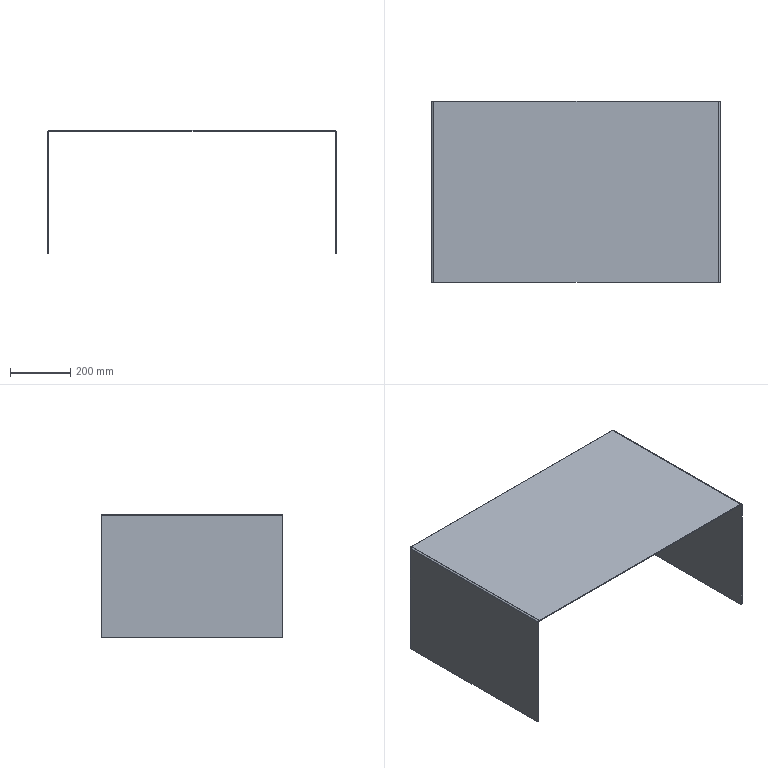Part | SolidWorks | features FlatPattern 1, ICE 1, SMBaseFlange 1, SheetMetal 1 | 1 solid | 26 faces | box 956 x 600 x 410 mm | volume 3179024 mm3 | plane 18 | cylinder 8 | commonest cylinder face diameters 6 x6 12 x2
STEP:
#1=CARTESIAN_POINT('',(956.,0.,-407.));
#2=VERTEX_POINT('',#1);
#3=CARTESIAN_POINT('',(956.,3.,-410.));
#4=VERTEX_POINT('',#3);
#5=CARTESIAN_POINT('',(956.,3.,-407.));
#6=DIRECTION('',(1.,0.,0.));
#7=DIRECTION('',(0.,0.,1.));
#8=AXIS2_PLACEMENT_3D('',#5,#6,#7);
#9=CIRCLE('',#8,3.);
#10=EDGE_CURVE('',#2,#4,#9,.T.);
#11=ORIENTED_EDGE('',*,*,#10,.T.);
#12=CARTESIAN_POINT('',(956.,597.,-410.));
#13=VERTEX_POINT('',#12);
#14=CARTESIAN_POINT('',(956.,600.,-410.));
#15=DIRECTION('',(0.,-1.,0.));
#16=VECTOR('',#15,1000.);
#17=LINE('',#14,#16);
#18=EDGE_CURVE('',#13,#4,#17,.T.);
#19=ORIENTED_EDGE('',*,*,#18,.F.);
#20=CARTESIAN_POINT('',(956.,600.,-407.));
#21=VERTEX_POINT('',#20);
#22=CARTESIAN_POINT('',(956.,597.,-407.));
#23=DIRECTION('',(1.,0.,0.));
#24=DIRECTION('',(0.,0.,1.));
#25=AXIS2_PLACEMENT_3D('',#22,#23,#24);
#26=CIRCLE('',#25,3.);
#27=EDGE_CURVE('',#13,#21,#26,.T.);
#28=ORIENTED_EDGE('',*,*,#27,.T.);
#29=CARTESIAN_POINT('',(956.,600.,-6.));
#30=VERTEX_POINT('',#29);
#31=CARTESIAN_POINT('',(956.,600.,0.));
#32=DIRECTION('',(0.,0.,-1.));
#33=VECTOR('',#32,1000.);
#34=LINE('',#31,#33);
#35=EDGE_CURVE('',#30,#21,#34,.T.);
#36=ORIENTED_EDGE('',*,*,#35,.F.);
#37=CARTESIAN_POINT('',(956.,0.,-6.));
#38=VERTEX_POINT('',#37);
#39=CARTESIAN_POINT('',(956.,600.,-6.));
#40=DIRECTION('',(0.,-1.,0.));
#41=VECTOR('',#40,1000.);
#42=LINE('',#39,#41);
#43=EDGE_CURVE('',#30,#38,#42,.T.);
#44=ORIENTED_EDGE('',*,*,#43,.T.);
#45=CARTESIAN_POINT('',(956.,0.,0.));
#46=DIRECTION('',(0.,0.,-1.));
#47=VECTOR('',#46,1000.);
#48=LINE('',#45,#47);
#49=EDGE_CURVE('',#38,#2,#48,.T.);
#50=ORIENTED_EDGE('',*,*,#49,.T.);
#51=EDGE_LOOP('',(#11,#19,#28,#36,#44,#50));
#52=FACE_OUTER_BOUND('',#51,.T.);
#53=CARTESIAN_POINT('',(956.,600.,0.));
#54=DIRECTION('',(-1.,0.,0.));
#55=DIRECTION('',(0.,0.,1.));
#56=AXIS2_PLACEMENT_3D('',#53,#54,#55);
#57=PLANE('',#56);
#58=ADVANCED_FACE('',(#52),#57,.F.);
#59=CARTESIAN_POINT('',(953.,597.,-410.));
#60=VERTEX_POINT('',#59);
#61=CARTESIAN_POINT('',(953.,3.,-410.));
#62=VERTEX_POINT('',#61);
#63=CARTESIAN_POINT('',(953.,600.,-410.));
#64=DIRECTION('',(0.,-1.,0.));
#65=VECTOR('',#64,1000.);
#66=LINE('',#63,#65);
#67=EDGE_CURVE('',#60,#62,#66,.T.);
#68=ORIENTED_EDGE('',*,*,#67,.T.);
#69=CARTESIAN_POINT('',(953.,0.,-407.));
#70=VERTEX_POINT('',#69);
#71=CARTESIAN_POINT('',(953.,3.,-407.));
#72=DIRECTION('',(1.,0.,0.));
#73=DIRECTION('',(0.,0.,1.));
#74=AXIS2_PLACEMENT_3D('',#71,#72,#73);
#75=CIRCLE('',#74,3.);
#76=EDGE_CURVE('',#70,#62,#75,.T.);
#77=ORIENTED_EDGE('',*,*,#76,.F.);
#78=CARTESIAN_POINT('',(953.,0.,-6.));
#79=VERTEX_POINT('',#78);
#80=CARTESIAN_POINT('',(953.,0.,0.));
#81=DIRECTION('',(0.,0.,-1.));
#82=VECTOR('',#81,1000.);
#83=LINE('',#80,#82);
#84=EDGE_CURVE('',#79,#70,#83,.T.);
#85=ORIENTED_EDGE('',*,*,#84,.F.);
#86=CARTESIAN_POINT('',(953.,600.,-6.));
#87=VERTEX_POINT('',#86);
#88=CARTESIAN_POINT('',(953.,600.,-6.));
#89=DIRECTION('',(0.,-1.,0.));
#90=VECTOR('',#89,1000.);
#91=LINE('',#88,#90);
#92=EDGE_CURVE('',#87,#79,#91,.T.);
#93=ORIENTED_EDGE('',*,*,#92,.F.);
#94=CARTESIAN_POINT('',(953.,600.,-407.));
#95=VERTEX_POINT('',#94);
#96=CARTESIAN_POINT('',(953.,600.,0.));
#97=DIRECTION('',(0.,0.,-1.));
#98=VECTOR('',#97,1000.);
#99=LINE('',#96,#98);
#100=EDGE_CURVE('',#87,#95,#99,.T.);
#101=ORIENTED_EDGE('',*,*,#100,.T.);
#102=CARTESIAN_POINT('',(953.,597.,-407.));
#103=DIRECTION('',(1.,0.,0.));
#104=DIRECTION('',(0.,0.,1.));
#105=AXIS2_PLACEMENT_3D('',#102,#103,#104);
#106=CIRCLE('',#105,3.);
#107=EDGE_CURVE('',#60,#95,#106,.T.);
#108=ORIENTED_EDGE('',*,*,#107,.F.);
#109=EDGE_LOOP('',(#68,#77,#85,#93,#101,#108));
#110=FACE_OUTER_BOUND('',#109,.T.);
#111=CARTESIAN_POINT('',(953.,600.,0.));
#112=DIRECTION('',(-1.,0.,0.));
#113=DIRECTION('',(0.,0.,1.));
#114=AXIS2_PLACEMENT_3D('',#111,#112,#113);
#115=PLANE('',#114);
#116=ADVANCED_FACE('',(#110),#115,.T.);
#117=ORIENTED_EDGE('',*,*,#18,.T.);
#118=CARTESIAN_POINT('',(953.,3.,-410.));
#119=DIRECTION('',(1.,0.,0.));
#120=VECTOR('',#119,1000.);
#121=LINE('',#118,#120);
#122=EDGE_CURVE('',#62,#4,#121,.T.);
#123=ORIENTED_EDGE('',*,*,#122,.F.);
#124=ORIENTED_EDGE('',*,*,#67,.F.);
#125=CARTESIAN_POINT('',(953.,597.,-410.));
#126=DIRECTION('',(1.,0.,0.));
#127=VECTOR('',#126,1000.);
#128=LINE('',#125,#127);
#129=EDGE_CURVE('',#60,#13,#128,.T.);
#130=ORIENTED_EDGE('',*,*,#129,.T.);
#131=EDGE_LOOP('',(#117,#123,#124,#130));
#132=FACE_OUTER_BOUND('',#131,.T.);
#133=CARTESIAN_POINT('',(953.,600.,-410.));
#134=DIRECTION('',(0.,0.,-1.));
#135=DIRECTION('',(-1.,0.,0.));
#136=AXIS2_PLACEMENT_3D('',#133,#134,#135);
#137=PLANE('',#136);
#138=ADVANCED_FACE('',(#132),#137,.T.);
#139=CARTESIAN_POINT('',(3.,0.,-407.));
#140=VERTEX_POINT('',#139);
#141=CARTESIAN_POINT('',(3.,0.,-6.));
#142=VERTEX_POINT('',#141);
#143=CARTESIAN_POINT('',(3.,0.,0.));
#144=DIRECTION('',(0.,0.,1.));
#145=VECTOR('',#144,1000.);
#146=LINE('',#143,#145);
#147=EDGE_CURVE('',#140,#142,#146,.T.);
#148=ORIENTED_EDGE('',*,*,#147,.F.);
#149=CARTESIAN_POINT('',(3.,3.,-410.));
#150=VERTEX_POINT('',#149);
#151=CARTESIAN_POINT('',(3.,3.,-407.));
#152=DIRECTION('',(-1.,0.,0.));
#153=DIRECTION('',(0.,0.,-1.));
#154=AXIS2_PLACEMENT_3D('',#151,#152,#153);
#155=CIRCLE('',#154,3.);
#156=EDGE_CURVE('',#150,#140,#155,.T.);
#157=ORIENTED_EDGE('',*,*,#156,.F.);
#158=CARTESIAN_POINT('',(3.,597.,-410.));
#159=VERTEX_POINT('',#158);
#160=CARTESIAN_POINT('',(3.,600.,-410.));
#161=DIRECTION('',(0.,-1.,0.));
#162=VECTOR('',#161,1000.);
#163=LINE('',#160,#162);
#164=EDGE_CURVE('',#159,#150,#163,.T.);
#165=ORIENTED_EDGE('',*,*,#164,.F.);
#166=CARTESIAN_POINT('',(3.,600.,-407.));
#167=VERTEX_POINT('',#166);
#168=CARTESIAN_POINT('',(3.,597.,-407.));
#169=DIRECTION('',(-1.,0.,0.));
#170=DIRECTION('',(0.,0.,-1.));
#171=AXIS2_PLACEMENT_3D('',#168,#169,#170);
#172=CIRCLE('',#171,3.);
#173=EDGE_CURVE('',#167,#159,#172,.T.);
#174=ORIENTED_EDGE('',*,*,#173,.F.);
#175=CARTESIAN_POINT('',(3.,600.,-6.));
#176=VERTEX_POINT('',#175);
#177=CARTESIAN_POINT('',(3.,600.,0.));
#178=DIRECTION('',(0.,0.,1.));
#179=VECTOR('',#178,1000.);
#180=LINE('',#177,#179);
#181=EDGE_CURVE('',#167,#176,#180,.T.);
#182=ORIENTED_EDGE('',*,*,#181,.T.);
#183=CARTESIAN_POINT('',(3.,600.,-6.));
#184=DIRECTION('',(0.,-1.,0.));
#185=VECTOR('',#184,1000.);
#186=LINE('',#183,#185);
#187=EDGE_CURVE('',#176,#142,#186,.T.);
#188=ORIENTED_EDGE('',*,*,#187,.T.);
#189=EDGE_LOOP('',(#148,#157,#165,#174,#182,#188));
#190=FACE_OUTER_BOUND('',#189,.T.);
#191=CARTESIAN_POINT('',(3.,600.,0.));
#192=DIRECTION('',(1.,0.,0.));
#193=DIRECTION('',(0.,0.,-1.));
#194=AXIS2_PLACEMENT_3D('',#191,#192,#193);
#195=PLANE('',#194);
#196=ADVANCED_FACE('',(#190),#195,.T.);
#197=CARTESIAN_POINT('',(0.,3.,-410.));
#198=VERTEX_POINT('',#197);
#199=CARTESIAN_POINT('',(0.,0.,-407.));
#200=VERTEX_POINT('',#199);
#201=CARTESIAN_POINT('',(0.,3.,-407.));
#202=DIRECTION('',(-1.,0.,0.));
#203=DIRECTION('',(0.,0.,-1.));
#204=AXIS2_PLACEMENT_3D('',#201,#202,#203);
#205=CIRCLE('',#204,3.);
#206=EDGE_CURVE('',#198,#200,#205,.T.);
#207=ORIENTED_EDGE('',*,*,#206,.T.);
#208=CARTESIAN_POINT('',(0.,0.,-6.));
#209=VERTEX_POINT('',#208);
#210=CARTESIAN_POINT('',(0.,0.,0.));
#211=DIRECTION('',(0.,0.,1.));
#212=VECTOR('',#211,1000.);
#213=LINE('',#210,#212);
#214=EDGE_CURVE('',#200,#209,#213,.T.);
#215=ORIENTED_EDGE('',*,*,#214,.T.);
#216=CARTESIAN_POINT('',(0.,600.,-6.));
#217=VERTEX_POINT('',#216);
#218=CARTESIAN_POINT('',(0.,600.,-6.));
#219=DIRECTION('',(0.,-1.,0.));
#220=VECTOR('',#219,1000.);
#221=LINE('',#218,#220);
#222=EDGE_CURVE('',#217,#209,#221,.T.);
#223=ORIENTED_EDGE('',*,*,#222,.F.);
#224=CARTESIAN_POINT('',(0.,600.,-407.));
#225=VERTEX_POINT('',#224);
#226=CARTESIAN_POINT('',(0.,600.,0.));
#227=DIRECTION('',(0.,0.,1.));
#228=VECTOR('',#227,1000.);
#229=LINE('',#226,#228);
#230=EDGE_CURVE('',#225,#217,#229,.T.);
#231=ORIENTED_EDGE('',*,*,#230,.F.);
#232=CARTESIAN_POINT('',(0.,597.,-410.));
#233=VERTEX_POINT('',#232);
#234=CARTESIAN_POINT('',(0.,597.,-407.));
#235=DIRECTION('',(-1.,0.,0.));
#236=DIRECTION('',(0.,0.,-1.));
#237=AXIS2_PLACEMENT_3D('',#234,#235,#236);
#238=CIRCLE('',#237,3.);
#239=EDGE_CURVE('',#225,#233,#238,.T.);
#240=ORIENTED_EDGE('',*,*,#239,.T.);
#241=CARTESIAN_POINT('',(0.,600.,-410.));
#242=DIRECTION('',(0.,-1.,0.));
#243=VECTOR('',#242,1000.);
#244=LINE('',#241,#243);
#245=EDGE_CURVE('',#233,#198,#244,.T.);
#246=ORIENTED_EDGE('',*,*,#245,.T.);
#247=EDGE_LOOP('',(#207,#215,#223,#231,#240,#246));
#248=FACE_OUTER_BOUND('',#247,.T.);
#249=CARTESIAN_POINT('',(0.,600.,0.));
#250=DIRECTION('',(1.,0.,0.));
#251=DIRECTION('',(0.,0.,-1.));
#252=AXIS2_PLACEMENT_3D('',#249,#250,#251);
#253=PLANE('',#252);
#254=ADVANCED_FACE('',(#248),#253,.F.);
#255=ORIENTED_EDGE('',*,*,#35,.T.);
#256=CARTESIAN_POINT('',(953.,600.,-407.));
#257=DIRECTION('',(1.,0.,0.));
#258=VECTOR('',#257,1000.);
#259=LINE('',#256,#258);
#260=EDGE_CURVE('',#95,#21,#259,.T.);
#261=ORIENTED_EDGE('',*,*,#260,.F.);
#262=ORIENTED_EDGE('',*,*,#100,.F.);
#263=CARTESIAN_POINT('',(953.,600.,-6.));
#264=DIRECTION('',(1.,0.,0.));
#265=VECTOR('',#264,1000.);
#266=LINE('',#263,#265);
#267=EDGE_CURVE('',#87,#30,#266,.T.);
#268=ORIENTED_EDGE('',*,*,#267,.T.);
#269=EDGE_LOOP('',(#255,#261,#262,#268));
#270=FACE_OUTER_BOUND('',#269,.T.);
#271=CARTESIAN_POINT('',(950.,600.,-6.));
#272=DIRECTION('',(0.,1.,0.));
#273=DIRECTION('',(1.,0.,0.));
#274=AXIS2_PLACEMENT_3D('',#271,#272,#273);
#275=PLANE('',#274);
#276=ADVANCED_FACE('',(#270),#275,.T.);
#277=CARTESIAN_POINT('',(3.,3.,-410.));
#278=DIRECTION('',(-1.,0.,0.));
#279=VECTOR('',#278,1000.);
#280=LINE('',#277,#279);
#281=EDGE_CURVE('',#150,#198,#280,.T.);
#282=ORIENTED_EDGE('',*,*,#281,.T.);
#283=ORIENTED_EDGE('',*,*,#245,.F.);
#284=CARTESIAN_POINT('',(3.,597.,-410.));
#285=DIRECTION('',(-1.,0.,0.));
#286=VECTOR('',#285,1000.);
#287=LINE('',#284,#286);
#288=EDGE_CURVE('',#159,#233,#287,.T.);
#289=ORIENTED_EDGE('',*,*,#288,.F.);
#290=ORIENTED_EDGE('',*,*,#164,.T.);
#291=EDGE_LOOP('',(#282,#283,#289,#290));
#292=FACE_OUTER_BOUND('',#291,.T.);
#293=CARTESIAN_POINT('',(0.,600.,-410.));
#294=DIRECTION('',(0.,0.,-1.));
#295=DIRECTION('',(-1.,0.,0.));
#296=AXIS2_PLACEMENT_3D('',#293,#294,#295);
#297=PLANE('',#296);
#298=ADVANCED_FACE('',(#292),#297,.T.);
#299=CARTESIAN_POINT('',(0.,600.,-6.));
#300=DIRECTION('',(1.,0.,0.));
#301=VECTOR('',#300,1000.);
#302=LINE('',#299,#301);
#303=EDGE_CURVE('',#217,#176,#302,.T.);
#304=ORIENTED_EDGE('',*,*,#303,.F.);
#305=CARTESIAN_POINT('',(6.,600.,0.));
#306=VERTEX_POINT('',#305);
#307=CARTESIAN_POINT('',(6.,600.,-6.));
#308=DIRECTION('',(0.,1.,0.));
#309=DIRECTION('',(0.,0.,-1.));
#310=AXIS2_PLACEMENT_3D('',#307,#308,#309);
#311=CIRCLE('',#310,6.);
#312=EDGE_CURVE('',#217,#306,#311,.T.);
#313=ORIENTED_EDGE('',*,*,#312,.T.);
#314=CARTESIAN_POINT('',(6.,600.,-3.));
#315=VERTEX_POINT('',#314);
#316=CARTESIAN_POINT('',(6.,600.,-3.));
#317=DIRECTION('',(0.,0.,1.));
#318=VECTOR('',#317,1000.);
#319=LINE('',#316,#318);
#320=EDGE_CURVE('',#315,#306,#319,.T.);
#321=ORIENTED_EDGE('',*,*,#320,.F.);
#322=CARTESIAN_POINT('',(6.,600.,-6.));
#323=DIRECTION('',(0.,1.,0.));
#324=DIRECTION('',(1.,0.,0.));
#325=AXIS2_PLACEMENT_3D('',#322,#323,#324);
#326=CIRCLE('',#325,3.);
#327=EDGE_CURVE('',#176,#315,#326,.T.);
#328=ORIENTED_EDGE('',*,*,#327,.F.);
#329=EDGE_LOOP('',(#304,#313,#321,#328));
#330=FACE_OUTER_BOUND('',#329,.T.);
#331=CARTESIAN_POINT('',(0.,600.,-6.));
#332=DIRECTION('',(0.,1.,0.));
#333=DIRECTION('',(0.,0.,1.));
#334=AXIS2_PLACEMENT_3D('',#331,#332,#333);
#335=PLANE('',#334);
#336=ADVANCED_FACE('',(#330),#335,.T.);
#337=CARTESIAN_POINT('',(3.,600.,-407.));
#338=DIRECTION('',(-1.,0.,0.));
#339=VECTOR('',#338,1000.);
#340=LINE('',#337,#339);
#341=EDGE_CURVE('',#167,#225,#340,.T.);
#342=ORIENTED_EDGE('',*,*,#341,.T.);
#343=ORIENTED_EDGE('',*,*,#230,.T.);
#344=ORIENTED_EDGE('',*,*,#303,.T.);
#345=ORIENTED_EDGE('',*,*,#181,.F.);
#346=EDGE_LOOP('',(#342,#343,#344,#345));
#347=FACE_OUTER_BOUND('',#346,.T.);
#348=CARTESIAN_POINT('',(6.,600.,-3.));
#349=DIRECTION('',(0.,1.,0.));
#350=DIRECTION('',(0.,0.,1.));
#351=AXIS2_PLACEMENT_3D('',#348,#349,#350);
#352=PLANE('',#351);
#353=ADVANCED_FACE('',(#347),#352,.T.);
#354=CARTESIAN_POINT('',(6.,0.,0.));
#355=VERTEX_POINT('',#354);
#356=CARTESIAN_POINT('',(6.,0.,-3.));
#357=VERTEX_POINT('',#356);
#358=CARTESIAN_POINT('',(6.,0.,0.));
#359=DIRECTION('',(0.,0.,-1.));
#360=VECTOR('',#359,1000.);
#361=LINE('',#358,#360);
#362=EDGE_CURVE('',#355,#357,#361,.T.);
#363=ORIENTED_EDGE('',*,*,#362,.F.);
#364=CARTESIAN_POINT('',(6.,0.,-6.));
#365=DIRECTION('',(0.,1.,0.));
#366=DIRECTION('',(0.,0.,-1.));
#367=AXIS2_PLACEMENT_3D('',#364,#365,#366);
#368=CIRCLE('',#367,6.);
#369=EDGE_CURVE('',#209,#355,#368,.T.);
#370=ORIENTED_EDGE('',*,*,#369,.F.);
#371=CARTESIAN_POINT('',(3.,0.,-6.));
#372=DIRECTION('',(-1.,0.,0.));
#373=VECTOR('',#372,1000.);
#374=LINE('',#371,#373);
#375=EDGE_CURVE('',#142,#209,#374,.T.);
#376=ORIENTED_EDGE('',*,*,#375,.F.);
#377=CARTESIAN_POINT('',(6.,0.,-6.));
#378=DIRECTION('',(0.,1.,0.));
#379=DIRECTION('',(1.,0.,0.));
#380=AXIS2_PLACEMENT_3D('',#377,#378,#379);
#381=CIRCLE('',#380,3.);
#382=EDGE_CURVE('',#142,#357,#381,.T.);
#383=ORIENTED_EDGE('',*,*,#382,.T.);
#384=EDGE_LOOP('',(#363,#370,#376,#383));
#385=FACE_OUTER_BOUND('',#384,.T.);
#386=CARTESIAN_POINT('',(6.,0.,0.));
#387=DIRECTION('',(0.,-1.,0.));
#388=DIRECTION('',(0.,0.,-1.));
#389=AXIS2_PLACEMENT_3D('',#386,#387,#388);
#390=PLANE('',#389);
#391=ADVANCED_FACE('',(#385),#390,.T.);
#392=CARTESIAN_POINT('',(950.,0.,0.));
#393=VERTEX_POINT('',#392);
#394=CARTESIAN_POINT('',(0.,0.,0.));
#395=DIRECTION('',(1.,0.,0.));
#396=VECTOR('',#395,1000.);
#397=LINE('',#394,#396);
#398=EDGE_CURVE('',#355,#393,#397,.T.);
#399=ORIENTED_EDGE('',*,*,#398,.F.);
#400=ORIENTED_EDGE('',*,*,#362,.T.);
#401=CARTESIAN_POINT('',(950.,0.,-3.));
#402=VERTEX_POINT('',#401);
#403=CARTESIAN_POINT('',(0.,0.,-3.));
#404=DIRECTION('',(1.,0.,0.));
#405=VECTOR('',#404,1000.);
#406=LINE('',#403,#405);
#407=EDGE_CURVE('',#357,#402,#406,.T.);
#408=ORIENTED_EDGE('',*,*,#407,.T.);
#409=CARTESIAN_POINT('',(950.,0.,-3.));
#410=DIRECTION('',(0.,0.,1.));
#411=VECTOR('',#410,1000.);
#412=LINE('',#409,#411);
#413=EDGE_CURVE('',#402,#393,#412,.T.);
#414=ORIENTED_EDGE('',*,*,#413,.T.);
#415=EDGE_LOOP('',(#399,#400,#408,#414));
#416=FACE_OUTER_BOUND('',#415,.T.);
#417=CARTESIAN_POINT('',(3.,0.,-6.));
#418=DIRECTION('',(0.,-1.,0.));
#419=DIRECTION('',(0.,0.,-1.));
#420=AXIS2_PLACEMENT_3D('',#417,#418,#419);
#421=PLANE('',#420);
#422=ADVANCED_FACE('',(#416),#421,.T.);
#423=CARTESIAN_POINT('',(950.,600.,0.));
#424=VERTEX_POINT('',#423);
#425=CARTESIAN_POINT('',(950.,600.,-3.));
#426=VERTEX_POINT('',#425);
#427=CARTESIAN_POINT('',(950.,600.,0.));
#428=DIRECTION('',(0.,0.,-1.));
#429=VECTOR('',#428,1000.);
#430=LINE('',#427,#429);
#431=EDGE_CURVE('',#424,#426,#430,.T.);
#432=ORIENTED_EDGE('',*,*,#431,.F.);
#433=CARTESIAN_POINT('',(950.,600.,-6.));
#434=DIRECTION('',(0.,1.,0.));
#435=DIRECTION('',(0.,0.,-1.));
#436=AXIS2_PLACEMENT_3D('',#433,#434,#435);
#437=CIRCLE('',#436,6.);
#438=EDGE_CURVE('',#424,#30,#437,.T.);
#439=ORIENTED_EDGE('',*,*,#438,.T.);
#440=ORIENTED_EDGE('',*,*,#267,.F.);
#441=CARTESIAN_POINT('',(950.,600.,-6.));
#442=DIRECTION('',(0.,1.,0.));
#443=DIRECTION('',(1.,0.,0.));
#444=AXIS2_PLACEMENT_3D('',#441,#442,#443);
#445=CIRCLE('',#444,3.);
#446=EDGE_CURVE('',#426,#87,#445,.T.);
#447=ORIENTED_EDGE('',*,*,#446,.F.);
#448=EDGE_LOOP('',(#432,#439,#440,#447));
#449=FACE_OUTER_BOUND('',#448,.T.);
#450=CARTESIAN_POINT('',(950.,600.,0.));
#451=DIRECTION('',(0.,1.,0.));
#452=DIRECTION('',(0.,0.,1.));
#453=AXIS2_PLACEMENT_3D('',#450,#451,#452);
#454=PLANE('',#453);
#455=ADVANCED_FACE('',(#449),#454,.T.);
#456=CARTESIAN_POINT('',(0.,600.,0.));
#457=DIRECTION('',(1.,0.,0.));
#458=VECTOR('',#457,1000.);
#459=LINE('',#456,#458);
#460=EDGE_CURVE('',#306,#424,#459,.T.);
#461=ORIENTED_EDGE('',*,*,#460,.T.);
#462=ORIENTED_EDGE('',*,*,#431,.T.);
#463=CARTESIAN_POINT('',(0.,600.,-3.));
#464=DIRECTION('',(1.,0.,0.));
#465=VECTOR('',#464,1000.);
#466=LINE('',#463,#465);
#467=EDGE_CURVE('',#315,#426,#466,.T.);
#468=ORIENTED_EDGE('',*,*,#467,.F.);
#469=ORIENTED_EDGE('',*,*,#320,.T.);
#470=EDGE_LOOP('',(#461,#462,#468,#469));
#471=FACE_OUTER_BOUND('',#470,.T.);
#472=CARTESIAN_POINT('',(953.,600.,-6.));
#473=DIRECTION('',(0.,1.,0.));
#474=DIRECTION('',(0.,0.,1.));
#475=AXIS2_PLACEMENT_3D('',#472,#473,#474);
#476=PLANE('',#475);
#477=ADVANCED_FACE('',(#471),#476,.T.);
#478=CARTESIAN_POINT('',(956.,0.,-6.));
#479=DIRECTION('',(-1.,0.,0.));
#480=VECTOR('',#479,1000.);
#481=LINE('',#478,#480);
#482=EDGE_CURVE('',#38,#79,#481,.T.);
#483=ORIENTED_EDGE('',*,*,#482,.F.);
#484=CARTESIAN_POINT('',(950.,0.,-6.));
#485=DIRECTION('',(0.,1.,0.));
#486=DIRECTION('',(0.,0.,-1.));
#487=AXIS2_PLACEMENT_3D('',#484,#485,#486);
#488=CIRCLE('',#487,6.);
#489=EDGE_CURVE('',#393,#38,#488,.T.);
#490=ORIENTED_EDGE('',*,*,#489,.F.);
#491=ORIENTED_EDGE('',*,*,#413,.F.);
#492=CARTESIAN_POINT('',(950.,0.,-6.));
#493=DIRECTION('',(0.,1.,0.));
#494=DIRECTION('',(1.,0.,0.));
#495=AXIS2_PLACEMENT_3D('',#492,#493,#494);
#496=CIRCLE('',#495,3.);
#497=EDGE_CURVE('',#402,#79,#496,.T.);
#498=ORIENTED_EDGE('',*,*,#497,.T.);
#499=EDGE_LOOP('',(#483,#490,#491,#498));
#500=FACE_OUTER_BOUND('',#499,.T.);
#501=CARTESIAN_POINT('',(956.,0.,-6.));
#502=DIRECTION('',(0.,-1.,0.));
#503=DIRECTION('',(0.,0.,-1.));
#504=AXIS2_PLACEMENT_3D('',#501,#502,#503);
#505=PLANE('',#504);
#506=ADVANCED_FACE('',(#500),#505,.T.);
#507=CARTESIAN_POINT('',(953.,0.,-407.));
#508=DIRECTION('',(1.,0.,0.));
#509=VECTOR('',#508,1000.);
#510=LINE('',#507,#509);
#511=EDGE_CURVE('',#70,#2,#510,.T.);
#512=ORIENTED_EDGE('',*,*,#511,.T.);
#513=ORIENTED_EDGE('',*,*,#49,.F.);
#514=ORIENTED_EDGE('',*,*,#482,.T.);
#515=ORIENTED_EDGE('',*,*,#84,.T.);
#516=EDGE_LOOP('',(#512,#513,#514,#515));
#517=FACE_OUTER_BOUND('',#516,.T.);
#518=CARTESIAN_POINT('',(950.,0.,-3.));
#519=DIRECTION('',(0.,-1.,0.));
#520=DIRECTION('',(0.,0.,-1.));
#521=AXIS2_PLACEMENT_3D('',#518,#519,#520);
#522=PLANE('',#521);
#523=ADVANCED_FACE('',(#517),#522,.T.);
#524=ORIENTED_EDGE('',*,*,#497,.F.);
#525=CARTESIAN_POINT('',(950.,600.,-3.));
#526=DIRECTION('',(0.,-1.,0.));
#527=VECTOR('',#526,1000.);
#528=LINE('',#525,#527);
#529=EDGE_CURVE('',#426,#402,#528,.T.);
#530=ORIENTED_EDGE('',*,*,#529,.F.);
#531=ORIENTED_EDGE('',*,*,#446,.T.);
#532=ORIENTED_EDGE('',*,*,#92,.T.);
#533=EDGE_LOOP('',(#524,#530,#531,#532));
#534=FACE_OUTER_BOUND('',#533,.T.);
#535=CARTESIAN_POINT('',(950.,600.,-6.));
#536=DIRECTION('',(0.,-1.,0.));
#537=DIRECTION('',(0.,0.,-1.));
#538=AXIS2_PLACEMENT_3D('',#535,#536,#537);
#539=CYLINDRICAL_SURFACE('',#538,3.);
#540=ADVANCED_FACE('',(#534),#539,.F.);
#541=ORIENTED_EDGE('',*,*,#407,.F.);
#542=CARTESIAN_POINT('',(6.,600.,-3.));
#543=DIRECTION('',(0.,-1.,0.));
#544=VECTOR('',#543,1000.);
#545=LINE('',#542,#544);
#546=EDGE_CURVE('',#315,#357,#545,.T.);
#547=ORIENTED_EDGE('',*,*,#546,.F.);
#548=ORIENTED_EDGE('',*,*,#467,.T.);
#549=ORIENTED_EDGE('',*,*,#529,.T.);
#550=EDGE_LOOP('',(#541,#547,#548,#549));
#551=FACE_OUTER_BOUND('',#550,.T.);
#552=CARTESIAN_POINT('',(0.,600.,-3.));
#553=DIRECTION('',(0.,0.,-1.));
#554=DIRECTION('',(-1.,0.,0.));
#555=AXIS2_PLACEMENT_3D('',#552,#553,#554);
#556=PLANE('',#555);
#557=ADVANCED_FACE('',(#551),#556,.T.);
#558=ORIENTED_EDGE('',*,*,#382,.F.);
#559=ORIENTED_EDGE('',*,*,#187,.F.);
#560=ORIENTED_EDGE('',*,*,#327,.T.);
#561=ORIENTED_EDGE('',*,*,#546,.T.);
#562=EDGE_LOOP('',(#558,#559,#560,#561));
#563=FACE_OUTER_BOUND('',#562,.T.);
#564=CARTESIAN_POINT('',(6.,600.,-6.));
#565=DIRECTION('',(0.,-1.,0.));
#566=DIRECTION('',(0.,0.,-1.));
#567=AXIS2_PLACEMENT_3D('',#564,#565,#566);
#568=CYLINDRICAL_SURFACE('',#567,3.);
#569=ADVANCED_FACE('',(#563),#568,.F.);
#570=ORIENTED_EDGE('',*,*,#369,.T.);
#571=CARTESIAN_POINT('',(6.,600.,0.));
#572=DIRECTION('',(0.,-1.,0.));
#573=VECTOR('',#572,1000.);
#574=LINE('',#571,#573);
#575=EDGE_CURVE('',#306,#355,#574,.T.);
#576=ORIENTED_EDGE('',*,*,#575,.F.);
#577=ORIENTED_EDGE('',*,*,#312,.F.);
#578=ORIENTED_EDGE('',*,*,#222,.T.);
#579=EDGE_LOOP('',(#570,#576,#577,#578));
#580=FACE_OUTER_BOUND('',#579,.T.);
#581=CARTESIAN_POINT('',(6.,600.,-6.));
#582=DIRECTION('',(0.,-1.,0.));
#583=DIRECTION('',(0.,0.,-1.));
#584=AXIS2_PLACEMENT_3D('',#581,#582,#583);
#585=CYLINDRICAL_SURFACE('',#584,6.);
#586=ADVANCED_FACE('',(#580),#585,.T.);
#587=ORIENTED_EDGE('',*,*,#398,.T.);
#588=CARTESIAN_POINT('',(950.,600.,0.));
#589=DIRECTION('',(0.,-1.,0.));
#590=VECTOR('',#589,1000.);
#591=LINE('',#588,#590);
#592=EDGE_CURVE('',#424,#393,#591,.T.);
#593=ORIENTED_EDGE('',*,*,#592,.F.);
#594=ORIENTED_EDGE('',*,*,#460,.F.);
#595=ORIENTED_EDGE('',*,*,#575,.T.);
#596=EDGE_LOOP('',(#587,#593,#594,#595));
#597=FACE_OUTER_BOUND('',#596,.T.);
#598=CARTESIAN_POINT('',(0.,600.,0.));
#599=DIRECTION('',(0.,0.,-1.));
#600=DIRECTION('',(-1.,0.,0.));
#601=AXIS2_PLACEMENT_3D('',#598,#599,#600);
#602=PLANE('',#601);
#603=ADVANCED_FACE('',(#597),#602,.F.);
#604=ORIENTED_EDGE('',*,*,#489,.T.);
#605=ORIENTED_EDGE('',*,*,#43,.F.);
#606=ORIENTED_EDGE('',*,*,#438,.F.);
#607=ORIENTED_EDGE('',*,*,#592,.T.);
#608=EDGE_LOOP('',(#604,#605,#606,#607));
#609=FACE_OUTER_BOUND('',#608,.T.);
#610=CARTESIAN_POINT('',(950.,600.,-6.));
#611=DIRECTION('',(0.,-1.,0.));
#612=DIRECTION('',(0.,0.,-1.));
#613=AXIS2_PLACEMENT_3D('',#610,#611,#612);
#614=CYLINDRICAL_SURFACE('',#613,6.);
#615=ADVANCED_FACE('',(#609),#614,.T.);
#616=ORIENTED_EDGE('',*,*,#214,.F.);
#617=CARTESIAN_POINT('',(3.,0.,-407.));
#618=DIRECTION('',(-1.,0.,0.));
#619=VECTOR('',#618,1000.);
#620=LINE('',#617,#619);
#621=EDGE_CURVE('',#140,#200,#620,.T.);
#622=ORIENTED_EDGE('',*,*,#621,.F.);
#623=ORIENTED_EDGE('',*,*,#147,.T.);
#624=ORIENTED_EDGE('',*,*,#375,.T.);
#625=EDGE_LOOP('',(#616,#622,#623,#624));
#626=FACE_OUTER_BOUND('',#625,.T.);
#627=CARTESIAN_POINT('',(950.,0.,-6.));
#628=DIRECTION('',(0.,1.,0.));
#629=DIRECTION('',(1.,0.,0.));
#630=AXIS2_PLACEMENT_3D('',#627,#628,#629);
#631=PLANE('',#630);
#632=ADVANCED_FACE('',(#626),#631,.F.);
#633=ORIENTED_EDGE('',*,*,#173,.T.);
#634=ORIENTED_EDGE('',*,*,#288,.T.);
#635=ORIENTED_EDGE('',*,*,#239,.F.);
#636=ORIENTED_EDGE('',*,*,#341,.F.);
#637=EDGE_LOOP('',(#633,#634,#635,#636));
#638=FACE_OUTER_BOUND('',#637,.T.);
#639=CARTESIAN_POINT('',(3.,597.,-407.));
#640=DIRECTION('',(1.,0.,0.));
#641=DIRECTION('',(0.,0.,-1.));
#642=AXIS2_PLACEMENT_3D('',#639,#640,#641);
#643=CYLINDRICAL_SURFACE('',#642,3.);
#644=ADVANCED_FACE('',(#638),#643,.T.);
#645=ORIENTED_EDGE('',*,*,#107,.T.);
#646=ORIENTED_EDGE('',*,*,#260,.T.);
#647=ORIENTED_EDGE('',*,*,#27,.F.);
#648=ORIENTED_EDGE('',*,*,#129,.F.);
#649=EDGE_LOOP('',(#645,#646,#647,#648));
#650=FACE_OUTER_BOUND('',#649,.T.);
#651=CARTESIAN_POINT('',(953.,597.,-407.));
#652=DIRECTION('',(-1.,0.,0.));
#653=DIRECTION('',(0.,0.,1.));
#654=AXIS2_PLACEMENT_3D('',#651,#652,#653);
#655=CYLINDRICAL_SURFACE('',#654,3.);
#656=ADVANCED_FACE('',(#650),#655,.T.);
#657=ORIENTED_EDGE('',*,*,#156,.T.);
#658=ORIENTED_EDGE('',*,*,#621,.T.);
#659=ORIENTED_EDGE('',*,*,#206,.F.);
#660=ORIENTED_EDGE('',*,*,#281,.F.);
#661=EDGE_LOOP('',(#657,#658,#659,#660));
#662=FACE_OUTER_BOUND('',#661,.T.);
#663=CARTESIAN_POINT('',(3.,3.,-407.));
#664=DIRECTION('',(1.,0.,0.));
#665=DIRECTION('',(0.,0.,-1.));
#666=AXIS2_PLACEMENT_3D('',#663,#664,#665);
#667=CYLINDRICAL_SURFACE('',#666,3.);
#668=ADVANCED_FACE('',(#662),#667,.T.);
#669=ORIENTED_EDGE('',*,*,#76,.T.);
#670=ORIENTED_EDGE('',*,*,#122,.T.);
#671=ORIENTED_EDGE('',*,*,#10,.F.);
#672=ORIENTED_EDGE('',*,*,#511,.F.);
#673=EDGE_LOOP('',(#669,#670,#671,#672));
#674=FACE_OUTER_BOUND('',#673,.T.);
#675=CARTESIAN_POINT('',(953.,3.,-407.));
#676=DIRECTION('',(-1.,0.,0.));
#677=DIRECTION('',(0.,0.,1.));
#678=AXIS2_PLACEMENT_3D('',#675,#676,#677);
#679=CYLINDRICAL_SURFACE('',#678,3.);
#680=ADVANCED_FACE('',(#674),#679,.T.);
#681=CLOSED_SHELL('',(#58,#116,#138,#196,#254,#276,#298,#336,#353,#391,#422,#455,#477,#506,#523,#540,#557,#569,#586,#603,#615,#632,#644,#656,#668,#680));
#682=MANIFOLD_SOLID_BREP('',#681);
#683=CARTESIAN_POINT('',(0.,0.,0.));
#684=DIRECTION('',(0.,0.,1.));
#685=DIRECTION('',(1.,0.,0.));
#686=AXIS2_PLACEMENT_3D('',#683,#684,#685);
#687=(LENGTH_UNIT()NAMED_UNIT(*)SI_UNIT(.MILLI.,.METRE.));
#688=UNCERTAINTY_MEASURE_WITH_UNIT(LENGTH_MEASURE(0.00001),#687,'','');
#689=(NAMED_UNIT(*)PLANE_ANGLE_UNIT()SI_UNIT($,.RADIAN.));
#690=(NAMED_UNIT(*)SI_UNIT($,.STERADIAN.)SOLID_ANGLE_UNIT());
#691=(GEOMETRIC_REPRESENTATION_CONTEXT(3)GLOBAL_UNCERTAINTY_ASSIGNED_CONTEXT((#688))GLOBAL_UNIT_ASSIGNED_CONTEXT((#687,#689,#690))REPRESENTATION_CONTEXT('',''));
#692=ADVANCED_BREP_SHAPE_REPRESENTATION('',(#682,#686),#691);